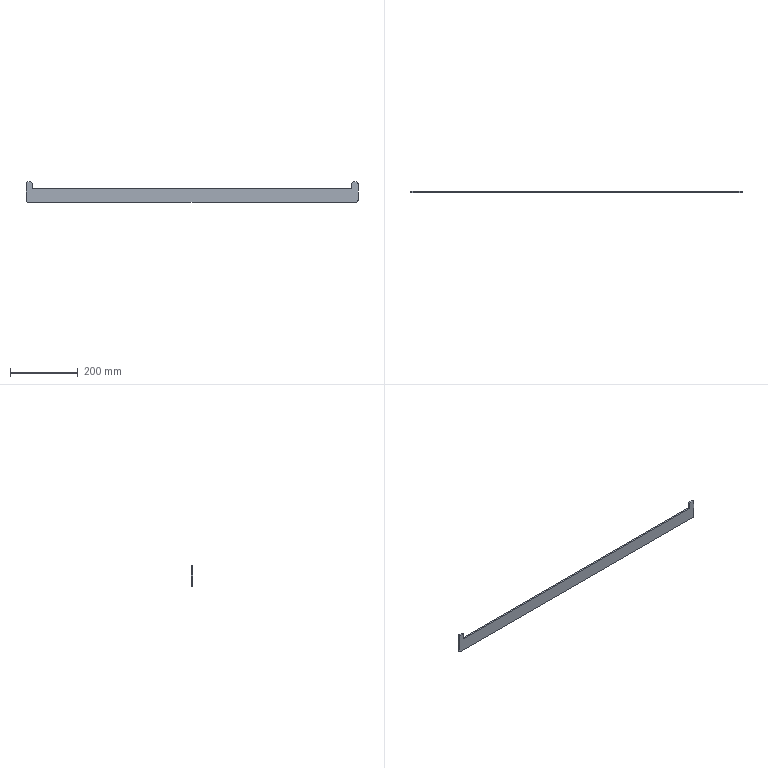Part | SolidWorks | features ICE 3, Fillet 2, FlatPattern 1, SMBaseFlange 1, SheetMetal 1 | 1 solid | 16 faces | box 980 x 5 x 60 mm | volume 199439 mm3 | plane 10 | cylinder 6 | commonest cylinder face diameters 10 x6
STEP:
#1=CARTESIAN_POINT('',(-472.,-5.,20.));
#2=VERTEX_POINT('',#1);
#3=CARTESIAN_POINT('',(-472.,0.,20.));
#4=VERTEX_POINT('',#3);
#5=CARTESIAN_POINT('',(-472.,-31.907,20.));
#6=DIRECTION('',(0.,1.,0.));
#7=VECTOR('',#6,1000.);
#8=LINE('',#5,#7);
#9=EDGE_CURVE('',#2,#4,#8,.T.);
#10=ORIENTED_EDGE('',*,*,#9,.F.);
#11=CARTESIAN_POINT('',(472.,-5.,20.));
#12=VERTEX_POINT('',#11);
#13=CARTESIAN_POINT('',(-490.,-5.,20.));
#14=DIRECTION('',(1.,0.,0.));
#15=VECTOR('',#14,1000.);
#16=LINE('',#13,#15);
#17=EDGE_CURVE('',#2,#12,#16,.T.);
#18=ORIENTED_EDGE('',*,*,#17,.T.);
#19=CARTESIAN_POINT('',(472.,0.,20.));
#20=VERTEX_POINT('',#19);
#21=CARTESIAN_POINT('',(472.,-5.,20.));
#22=DIRECTION('',(0.,1.,0.));
#23=VECTOR('',#22,1000.);
#24=LINE('',#21,#23);
#25=EDGE_CURVE('',#12,#20,#24,.T.);
#26=ORIENTED_EDGE('',*,*,#25,.T.);
#27=CARTESIAN_POINT('',(-490.,0.,20.));
#28=DIRECTION('',(1.,0.,0.));
#29=VECTOR('',#28,1000.);
#30=LINE('',#27,#29);
#31=EDGE_CURVE('',#4,#20,#30,.T.);
#32=ORIENTED_EDGE('',*,*,#31,.F.);
#33=EDGE_LOOP('',(#10,#18,#26,#32));
#34=FACE_OUTER_BOUND('',#33,.T.);
#35=CARTESIAN_POINT('',(-490.,-5.,20.));
#36=DIRECTION('',(0.,0.,1.));
#37=DIRECTION('',(1.,0.,0.));
#38=AXIS2_PLACEMENT_3D('',#35,#36,#37);
#39=PLANE('',#38);
#40=ADVANCED_FACE('',(#34),#39,.T.);
#41=CARTESIAN_POINT('',(490.,-5.,35.));
#42=VERTEX_POINT('',#41);
#43=CARTESIAN_POINT('',(490.,-5.,-15.));
#44=VERTEX_POINT('',#43);
#45=CARTESIAN_POINT('',(490.,-5.,20.));
#46=DIRECTION('',(0.,0.,-1.));
#47=VECTOR('',#46,1000.);
#48=LINE('',#45,#47);
#49=EDGE_CURVE('',#42,#44,#48,.T.);
#50=ORIENTED_EDGE('',*,*,#49,.T.);
#51=CARTESIAN_POINT('',(490.,0.,-15.));
#52=VERTEX_POINT('',#51);
#53=CARTESIAN_POINT('',(490.,-5.,-15.));
#54=DIRECTION('',(0.,1.,0.));
#55=VECTOR('',#54,1000.);
#56=LINE('',#53,#55);
#57=EDGE_CURVE('',#44,#52,#56,.T.);
#58=ORIENTED_EDGE('',*,*,#57,.T.);
#59=CARTESIAN_POINT('',(490.,0.,35.));
#60=VERTEX_POINT('',#59);
#61=CARTESIAN_POINT('',(490.,0.,20.));
#62=DIRECTION('',(0.,0.,-1.));
#63=VECTOR('',#62,1000.);
#64=LINE('',#61,#63);
#65=EDGE_CURVE('',#60,#52,#64,.T.);
#66=ORIENTED_EDGE('',*,*,#65,.F.);
#67=CARTESIAN_POINT('',(490.,-5.,35.));
#68=DIRECTION('',(0.,-1.,0.));
#69=VECTOR('',#68,1000.);
#70=LINE('',#67,#69);
#71=EDGE_CURVE('',#60,#42,#70,.T.);
#72=ORIENTED_EDGE('',*,*,#71,.T.);
#73=EDGE_LOOP('',(#50,#58,#66,#72));
#74=FACE_OUTER_BOUND('',#73,.T.);
#75=CARTESIAN_POINT('',(490.,-5.,20.));
#76=DIRECTION('',(1.,0.,0.));
#77=DIRECTION('',(0.,0.,-1.));
#78=AXIS2_PLACEMENT_3D('',#75,#76,#77);
#79=PLANE('',#78);
#80=ADVANCED_FACE('',(#74),#79,.T.);
#81=CARTESIAN_POINT('',(-490.,-5.,-15.));
#82=VERTEX_POINT('',#81);
#83=CARTESIAN_POINT('',(-490.,-5.,35.));
#84=VERTEX_POINT('',#83);
#85=CARTESIAN_POINT('',(-490.,-5.,20.));
#86=DIRECTION('',(0.,0.,1.));
#87=VECTOR('',#86,1000.);
#88=LINE('',#85,#87);
#89=EDGE_CURVE('',#82,#84,#88,.T.);
#90=ORIENTED_EDGE('',*,*,#89,.T.);
#91=CARTESIAN_POINT('',(-490.,0.,35.));
#92=VERTEX_POINT('',#91);
#93=CARTESIAN_POINT('',(-490.,-5.,35.));
#94=DIRECTION('',(0.,1.,0.));
#95=VECTOR('',#94,1000.);
#96=LINE('',#93,#95);
#97=EDGE_CURVE('',#84,#92,#96,.T.);
#98=ORIENTED_EDGE('',*,*,#97,.T.);
#99=CARTESIAN_POINT('',(-490.,0.,-15.));
#100=VERTEX_POINT('',#99);
#101=CARTESIAN_POINT('',(-490.,0.,20.));
#102=DIRECTION('',(0.,0.,1.));
#103=VECTOR('',#102,1000.);
#104=LINE('',#101,#103);
#105=EDGE_CURVE('',#100,#92,#104,.T.);
#106=ORIENTED_EDGE('',*,*,#105,.F.);
#107=CARTESIAN_POINT('',(-490.,-5.,-15.));
#108=DIRECTION('',(0.,-1.,0.));
#109=VECTOR('',#108,1000.);
#110=LINE('',#107,#109);
#111=EDGE_CURVE('',#100,#82,#110,.T.);
#112=ORIENTED_EDGE('',*,*,#111,.T.);
#113=EDGE_LOOP('',(#90,#98,#106,#112));
#114=FACE_OUTER_BOUND('',#113,.T.);
#115=CARTESIAN_POINT('',(-490.,-5.,20.));
#116=DIRECTION('',(-1.,0.,0.));
#117=DIRECTION('',(0.,0.,1.));
#118=AXIS2_PLACEMENT_3D('',#115,#116,#117);
#119=PLANE('',#118);
#120=ADVANCED_FACE('',(#114),#119,.T.);
#121=CARTESIAN_POINT('',(485.,0.,-20.));
#122=VERTEX_POINT('',#121);
#123=CARTESIAN_POINT('',(-485.,0.,-20.));
#124=VERTEX_POINT('',#123);
#125=CARTESIAN_POINT('',(-490.,0.,-20.));
#126=DIRECTION('',(-1.,0.,0.));
#127=VECTOR('',#126,1000.);
#128=LINE('',#125,#127);
#129=EDGE_CURVE('',#122,#124,#128,.T.);
#130=ORIENTED_EDGE('',*,*,#129,.F.);
#131=CARTESIAN_POINT('',(485.,-5.,-20.));
#132=VERTEX_POINT('',#131);
#133=CARTESIAN_POINT('',(485.,-5.,-20.));
#134=DIRECTION('',(0.,-1.,0.));
#135=VECTOR('',#134,1000.);
#136=LINE('',#133,#135);
#137=EDGE_CURVE('',#122,#132,#136,.T.);
#138=ORIENTED_EDGE('',*,*,#137,.T.);
#139=CARTESIAN_POINT('',(-485.,-5.,-20.));
#140=VERTEX_POINT('',#139);
#141=CARTESIAN_POINT('',(-490.,-5.,-20.));
#142=DIRECTION('',(-1.,0.,0.));
#143=VECTOR('',#142,1000.);
#144=LINE('',#141,#143);
#145=EDGE_CURVE('',#132,#140,#144,.T.);
#146=ORIENTED_EDGE('',*,*,#145,.T.);
#147=CARTESIAN_POINT('',(-485.,-5.,-20.));
#148=DIRECTION('',(0.,1.,0.));
#149=VECTOR('',#148,1000.);
#150=LINE('',#147,#149);
#151=EDGE_CURVE('',#140,#124,#150,.T.);
#152=ORIENTED_EDGE('',*,*,#151,.T.);
#153=EDGE_LOOP('',(#130,#138,#146,#152));
#154=FACE_OUTER_BOUND('',#153,.T.);
#155=CARTESIAN_POINT('',(-490.,-5.,-20.));
#156=DIRECTION('',(0.,0.,-1.));
#157=DIRECTION('',(-1.,0.,0.));
#158=AXIS2_PLACEMENT_3D('',#155,#156,#157);
#159=PLANE('',#158);
#160=ADVANCED_FACE('',(#154),#159,.T.);
#161=CARTESIAN_POINT('',(-472.,-5.,35.));
#162=VERTEX_POINT('',#161);
#163=CARTESIAN_POINT('',(-472.,-5.,20.));
#164=DIRECTION('',(0.,0.,-1.));
#165=VECTOR('',#164,1000.);
#166=LINE('',#163,#165);
#167=EDGE_CURVE('',#162,#2,#166,.T.);
#168=ORIENTED_EDGE('',*,*,#167,.F.);
#169=CARTESIAN_POINT('',(-477.,-5.,40.));
#170=VERTEX_POINT('',#169);
#171=CARTESIAN_POINT('',(-477.,-5.,35.));
#172=DIRECTION('',(0.,-1.,0.));
#173=DIRECTION('',(0.,0.,-1.));
#174=AXIS2_PLACEMENT_3D('',#171,#172,#173);
#175=CIRCLE('',#174,5.);
#176=EDGE_CURVE('',#162,#170,#175,.T.);
#177=ORIENTED_EDGE('',*,*,#176,.T.);
#178=CARTESIAN_POINT('',(-485.,-5.,40.));
#179=VERTEX_POINT('',#178);
#180=CARTESIAN_POINT('',(-490.,-5.,40.));
#181=DIRECTION('',(1.,0.,0.));
#182=VECTOR('',#181,1000.);
#183=LINE('',#180,#182);
#184=EDGE_CURVE('',#179,#170,#183,.T.);
#185=ORIENTED_EDGE('',*,*,#184,.F.);
#186=CARTESIAN_POINT('',(-485.,-5.,35.));
#187=DIRECTION('',(0.,-1.,0.));
#188=DIRECTION('',(0.,0.,-1.));
#189=AXIS2_PLACEMENT_3D('',#186,#187,#188);
#190=CIRCLE('',#189,5.);
#191=EDGE_CURVE('',#179,#84,#190,.T.);
#192=ORIENTED_EDGE('',*,*,#191,.T.);
#193=ORIENTED_EDGE('',*,*,#89,.F.);
#194=CARTESIAN_POINT('',(-485.,-5.,-15.));
#195=DIRECTION('',(0.,-1.,0.));
#196=DIRECTION('',(0.,0.,-1.));
#197=AXIS2_PLACEMENT_3D('',#194,#195,#196);
#198=CIRCLE('',#197,5.);
#199=EDGE_CURVE('',#82,#140,#198,.T.);
#200=ORIENTED_EDGE('',*,*,#199,.T.);
#201=ORIENTED_EDGE('',*,*,#145,.F.);
#202=CARTESIAN_POINT('',(485.,-5.,-15.));
#203=DIRECTION('',(0.,-1.,0.));
#204=DIRECTION('',(0.,0.,-1.));
#205=AXIS2_PLACEMENT_3D('',#202,#203,#204);
#206=CIRCLE('',#205,5.);
#207=EDGE_CURVE('',#132,#44,#206,.T.);
#208=ORIENTED_EDGE('',*,*,#207,.T.);
#209=ORIENTED_EDGE('',*,*,#49,.F.);
#210=CARTESIAN_POINT('',(485.,-5.,40.));
#211=VERTEX_POINT('',#210);
#212=CARTESIAN_POINT('',(485.,-5.,35.));
#213=DIRECTION('',(0.,-1.,0.));
#214=DIRECTION('',(0.,0.,-1.));
#215=AXIS2_PLACEMENT_3D('',#212,#213,#214);
#216=CIRCLE('',#215,5.);
#217=EDGE_CURVE('',#42,#211,#216,.T.);
#218=ORIENTED_EDGE('',*,*,#217,.T.);
#219=CARTESIAN_POINT('',(477.,-5.,40.));
#220=VERTEX_POINT('',#219);
#221=CARTESIAN_POINT('',(490.,-5.,40.));
#222=DIRECTION('',(1.,0.,0.));
#223=VECTOR('',#222,1000.);
#224=LINE('',#221,#223);
#225=EDGE_CURVE('',#220,#211,#224,.T.);
#226=ORIENTED_EDGE('',*,*,#225,.F.);
#227=CARTESIAN_POINT('',(472.,-5.,35.));
#228=VERTEX_POINT('',#227);
#229=CARTESIAN_POINT('',(477.,-5.,35.));
#230=DIRECTION('',(0.,-1.,0.));
#231=DIRECTION('',(0.,0.,-1.));
#232=AXIS2_PLACEMENT_3D('',#229,#230,#231);
#233=CIRCLE('',#232,5.);
#234=EDGE_CURVE('',#220,#228,#233,.T.);
#235=ORIENTED_EDGE('',*,*,#234,.T.);
#236=CARTESIAN_POINT('',(472.,-5.,20.));
#237=DIRECTION('',(0.,0.,1.));
#238=VECTOR('',#237,1000.);
#239=LINE('',#236,#238);
#240=EDGE_CURVE('',#12,#228,#239,.T.);
#241=ORIENTED_EDGE('',*,*,#240,.F.);
#242=ORIENTED_EDGE('',*,*,#17,.F.);
#243=EDGE_LOOP('',(#168,#177,#185,#192,#193,#200,#201,#208,#209,#218,#226,#235,#241,#242));
#244=FACE_OUTER_BOUND('',#243,.T.);
#245=CARTESIAN_POINT('',(0.,-5.,0.));
#246=DIRECTION('',(0.,-1.,0.));
#247=DIRECTION('',(0.,0.,-1.));
#248=AXIS2_PLACEMENT_3D('',#245,#246,#247);
#249=PLANE('',#248);
#250=ADVANCED_FACE('',(#244),#249,.T.);
#251=CARTESIAN_POINT('',(-485.,0.,40.));
#252=VERTEX_POINT('',#251);
#253=CARTESIAN_POINT('',(-477.,0.,40.));
#254=VERTEX_POINT('',#253);
#255=CARTESIAN_POINT('',(-490.,0.,40.));
#256=DIRECTION('',(1.,0.,0.));
#257=VECTOR('',#256,1000.);
#258=LINE('',#255,#257);
#259=EDGE_CURVE('',#252,#254,#258,.T.);
#260=ORIENTED_EDGE('',*,*,#259,.T.);
#261=CARTESIAN_POINT('',(-472.,0.,35.));
#262=VERTEX_POINT('',#261);
#263=CARTESIAN_POINT('',(-477.,0.,35.));
#264=DIRECTION('',(0.,1.,0.));
#265=DIRECTION('',(0.,0.,-1.));
#266=AXIS2_PLACEMENT_3D('',#263,#264,#265);
#267=CIRCLE('',#266,5.);
#268=EDGE_CURVE('',#254,#262,#267,.T.);
#269=ORIENTED_EDGE('',*,*,#268,.T.);
#270=CARTESIAN_POINT('',(-472.,0.,20.));
#271=DIRECTION('',(0.,0.,-1.));
#272=VECTOR('',#271,1000.);
#273=LINE('',#270,#272);
#274=EDGE_CURVE('',#262,#4,#273,.T.);
#275=ORIENTED_EDGE('',*,*,#274,.T.);
#276=ORIENTED_EDGE('',*,*,#31,.T.);
#277=CARTESIAN_POINT('',(472.,0.,35.));
#278=VERTEX_POINT('',#277);
#279=CARTESIAN_POINT('',(472.,0.,20.));
#280=DIRECTION('',(0.,0.,1.));
#281=VECTOR('',#280,1000.);
#282=LINE('',#279,#281);
#283=EDGE_CURVE('',#20,#278,#282,.T.);
#284=ORIENTED_EDGE('',*,*,#283,.T.);
#285=CARTESIAN_POINT('',(477.,0.,40.));
#286=VERTEX_POINT('',#285);
#287=CARTESIAN_POINT('',(477.,0.,35.));
#288=DIRECTION('',(0.,1.,0.));
#289=DIRECTION('',(0.,0.,-1.));
#290=AXIS2_PLACEMENT_3D('',#287,#288,#289);
#291=CIRCLE('',#290,5.);
#292=EDGE_CURVE('',#278,#286,#291,.T.);
#293=ORIENTED_EDGE('',*,*,#292,.T.);
#294=CARTESIAN_POINT('',(485.,0.,40.));
#295=VERTEX_POINT('',#294);
#296=CARTESIAN_POINT('',(490.,0.,40.));
#297=DIRECTION('',(1.,0.,0.));
#298=VECTOR('',#297,1000.);
#299=LINE('',#296,#298);
#300=EDGE_CURVE('',#286,#295,#299,.T.);
#301=ORIENTED_EDGE('',*,*,#300,.T.);
#302=CARTESIAN_POINT('',(485.,0.,35.));
#303=DIRECTION('',(0.,1.,0.));
#304=DIRECTION('',(0.,0.,-1.));
#305=AXIS2_PLACEMENT_3D('',#302,#303,#304);
#306=CIRCLE('',#305,5.);
#307=EDGE_CURVE('',#295,#60,#306,.T.);
#308=ORIENTED_EDGE('',*,*,#307,.T.);
#309=ORIENTED_EDGE('',*,*,#65,.T.);
#310=CARTESIAN_POINT('',(485.,0.,-15.));
#311=DIRECTION('',(0.,1.,0.));
#312=DIRECTION('',(0.,0.,-1.));
#313=AXIS2_PLACEMENT_3D('',#310,#311,#312);
#314=CIRCLE('',#313,5.);
#315=EDGE_CURVE('',#52,#122,#314,.T.);
#316=ORIENTED_EDGE('',*,*,#315,.T.);
#317=ORIENTED_EDGE('',*,*,#129,.T.);
#318=CARTESIAN_POINT('',(-485.,0.,-15.));
#319=DIRECTION('',(0.,1.,0.));
#320=DIRECTION('',(0.,0.,-1.));
#321=AXIS2_PLACEMENT_3D('',#318,#319,#320);
#322=CIRCLE('',#321,5.);
#323=EDGE_CURVE('',#124,#100,#322,.T.);
#324=ORIENTED_EDGE('',*,*,#323,.T.);
#325=ORIENTED_EDGE('',*,*,#105,.T.);
#326=CARTESIAN_POINT('',(-485.,0.,35.));
#327=DIRECTION('',(0.,1.,0.));
#328=DIRECTION('',(0.,0.,-1.));
#329=AXIS2_PLACEMENT_3D('',#326,#327,#328);
#330=CIRCLE('',#329,5.);
#331=EDGE_CURVE('',#92,#252,#330,.T.);
#332=ORIENTED_EDGE('',*,*,#331,.T.);
#333=EDGE_LOOP('',(#260,#269,#275,#276,#284,#293,#301,#308,#309,#316,#317,#324,#325,#332));
#334=FACE_OUTER_BOUND('',#333,.T.);
#335=CARTESIAN_POINT('',(0.,0.,0.));
#336=DIRECTION('',(0.,-1.,0.));
#337=DIRECTION('',(0.,0.,-1.));
#338=AXIS2_PLACEMENT_3D('',#335,#336,#337);
#339=PLANE('',#338);
#340=ADVANCED_FACE('',(#334),#339,.F.);
#341=ORIENTED_EDGE('',*,*,#225,.T.);
#342=CARTESIAN_POINT('',(485.,-5.,40.));
#343=DIRECTION('',(0.,1.,0.));
#344=VECTOR('',#343,1000.);
#345=LINE('',#342,#344);
#346=EDGE_CURVE('',#211,#295,#345,.T.);
#347=ORIENTED_EDGE('',*,*,#346,.T.);
#348=ORIENTED_EDGE('',*,*,#300,.F.);
#349=CARTESIAN_POINT('',(477.,-5.,40.));
#350=DIRECTION('',(0.,-1.,0.));
#351=VECTOR('',#350,1000.);
#352=LINE('',#349,#351);
#353=EDGE_CURVE('',#286,#220,#352,.T.);
#354=ORIENTED_EDGE('',*,*,#353,.T.);
#355=EDGE_LOOP('',(#341,#347,#348,#354));
#356=FACE_OUTER_BOUND('',#355,.T.);
#357=CARTESIAN_POINT('',(490.,-5.,40.));
#358=DIRECTION('',(0.,0.,1.));
#359=DIRECTION('',(1.,0.,0.));
#360=AXIS2_PLACEMENT_3D('',#357,#358,#359);
#361=PLANE('',#360);
#362=ADVANCED_FACE('',(#356),#361,.T.);
#363=ORIENTED_EDGE('',*,*,#240,.T.);
#364=CARTESIAN_POINT('',(472.,-5.,35.));
#365=DIRECTION('',(0.,1.,0.));
#366=VECTOR('',#365,1000.);
#367=LINE('',#364,#366);
#368=EDGE_CURVE('',#228,#278,#367,.T.);
#369=ORIENTED_EDGE('',*,*,#368,.T.);
#370=ORIENTED_EDGE('',*,*,#283,.F.);
#371=ORIENTED_EDGE('',*,*,#25,.F.);
#372=EDGE_LOOP('',(#363,#369,#370,#371));
#373=FACE_OUTER_BOUND('',#372,.T.);
#374=CARTESIAN_POINT('',(472.,-5.,20.));
#375=DIRECTION('',(-1.,0.,0.));
#376=DIRECTION('',(0.,0.,1.));
#377=AXIS2_PLACEMENT_3D('',#374,#375,#376);
#378=PLANE('',#377);
#379=ADVANCED_FACE('',(#373),#378,.T.);
#380=ORIENTED_EDGE('',*,*,#207,.F.);
#381=ORIENTED_EDGE('',*,*,#137,.F.);
#382=ORIENTED_EDGE('',*,*,#315,.F.);
#383=ORIENTED_EDGE('',*,*,#57,.F.);
#384=EDGE_LOOP('',(#380,#381,#382,#383));
#385=FACE_OUTER_BOUND('',#384,.T.);
#386=CARTESIAN_POINT('',(485.,-5.,-15.));
#387=DIRECTION('',(0.,1.,0.));
#388=DIRECTION('',(0.,0.,1.));
#389=AXIS2_PLACEMENT_3D('',#386,#387,#388);
#390=CYLINDRICAL_SURFACE('',#389,5.);
#391=ADVANCED_FACE('',(#385),#390,.T.);
#392=ORIENTED_EDGE('',*,*,#199,.F.);
#393=ORIENTED_EDGE('',*,*,#111,.F.);
#394=ORIENTED_EDGE('',*,*,#323,.F.);
#395=ORIENTED_EDGE('',*,*,#151,.F.);
#396=EDGE_LOOP('',(#392,#393,#394,#395));
#397=FACE_OUTER_BOUND('',#396,.T.);
#398=CARTESIAN_POINT('',(-485.,-5.,-15.));
#399=DIRECTION('',(0.,1.,0.));
#400=DIRECTION('',(0.,0.,1.));
#401=AXIS2_PLACEMENT_3D('',#398,#399,#400);
#402=CYLINDRICAL_SURFACE('',#401,5.);
#403=ADVANCED_FACE('',(#397),#402,.T.);
#404=ORIENTED_EDGE('',*,*,#217,.F.);
#405=ORIENTED_EDGE('',*,*,#71,.F.);
#406=ORIENTED_EDGE('',*,*,#307,.F.);
#407=ORIENTED_EDGE('',*,*,#346,.F.);
#408=EDGE_LOOP('',(#404,#405,#406,#407));
#409=FACE_OUTER_BOUND('',#408,.T.);
#410=CARTESIAN_POINT('',(485.,-5.,35.));
#411=DIRECTION('',(0.,1.,0.));
#412=DIRECTION('',(0.,0.,1.));
#413=AXIS2_PLACEMENT_3D('',#410,#411,#412);
#414=CYLINDRICAL_SURFACE('',#413,5.);
#415=ADVANCED_FACE('',(#409),#414,.T.);
#416=ORIENTED_EDGE('',*,*,#234,.F.);
#417=ORIENTED_EDGE('',*,*,#353,.F.);
#418=ORIENTED_EDGE('',*,*,#292,.F.);
#419=ORIENTED_EDGE('',*,*,#368,.F.);
#420=EDGE_LOOP('',(#416,#417,#418,#419));
#421=FACE_OUTER_BOUND('',#420,.T.);
#422=CARTESIAN_POINT('',(477.,-5.,35.));
#423=DIRECTION('',(0.,1.,0.));
#424=DIRECTION('',(0.,0.,1.));
#425=AXIS2_PLACEMENT_3D('',#422,#423,#424);
#426=CYLINDRICAL_SURFACE('',#425,5.);
#427=ADVANCED_FACE('',(#421),#426,.T.);
#428=ORIENTED_EDGE('',*,*,#184,.T.);
#429=CARTESIAN_POINT('',(-477.,-31.907,40.));
#430=DIRECTION('',(0.,1.,0.));
#431=VECTOR('',#430,1000.);
#432=LINE('',#429,#431);
#433=EDGE_CURVE('',#170,#254,#432,.T.);
#434=ORIENTED_EDGE('',*,*,#433,.T.);
#435=ORIENTED_EDGE('',*,*,#259,.F.);
#436=CARTESIAN_POINT('',(-485.,-31.907,40.));
#437=DIRECTION('',(0.,-1.,0.));
#438=VECTOR('',#437,1000.);
#439=LINE('',#436,#438);
#440=EDGE_CURVE('',#252,#179,#439,.T.);
#441=ORIENTED_EDGE('',*,*,#440,.T.);
#442=EDGE_LOOP('',(#428,#434,#435,#441));
#443=FACE_OUTER_BOUND('',#442,.T.);
#444=CARTESIAN_POINT('',(-490.,-31.907,40.));
#445=DIRECTION('',(0.,0.,1.));
#446=DIRECTION('',(1.,0.,0.));
#447=AXIS2_PLACEMENT_3D('',#444,#445,#446);
#448=PLANE('',#447);
#449=ADVANCED_FACE('',(#443),#448,.T.);
#450=ORIENTED_EDGE('',*,*,#274,.F.);
#451=CARTESIAN_POINT('',(-472.,-31.907,35.));
#452=DIRECTION('',(0.,-1.,0.));
#453=VECTOR('',#452,1000.);
#454=LINE('',#451,#453);
#455=EDGE_CURVE('',#262,#162,#454,.T.);
#456=ORIENTED_EDGE('',*,*,#455,.T.);
#457=ORIENTED_EDGE('',*,*,#167,.T.);
#458=ORIENTED_EDGE('',*,*,#9,.T.);
#459=EDGE_LOOP('',(#450,#456,#457,#458));
#460=FACE_OUTER_BOUND('',#459,.T.);
#461=CARTESIAN_POINT('',(-472.,-31.907,20.));
#462=DIRECTION('',(1.,0.,0.));
#463=DIRECTION('',(0.,0.,-1.));
#464=AXIS2_PLACEMENT_3D('',#461,#462,#463);
#465=PLANE('',#464);
#466=ADVANCED_FACE('',(#460),#465,.T.);
#467=ORIENTED_EDGE('',*,*,#176,.F.);
#468=ORIENTED_EDGE('',*,*,#455,.F.);
#469=ORIENTED_EDGE('',*,*,#268,.F.);
#470=ORIENTED_EDGE('',*,*,#433,.F.);
#471=EDGE_LOOP('',(#467,#468,#469,#470));
#472=FACE_OUTER_BOUND('',#471,.T.);
#473=CARTESIAN_POINT('',(-477.,-31.907,35.));
#474=DIRECTION('',(0.,1.,0.));
#475=DIRECTION('',(0.,0.,1.));
#476=AXIS2_PLACEMENT_3D('',#473,#474,#475);
#477=CYLINDRICAL_SURFACE('',#476,5.);
#478=ADVANCED_FACE('',(#472),#477,.T.);
#479=ORIENTED_EDGE('',*,*,#191,.F.);
#480=ORIENTED_EDGE('',*,*,#440,.F.);
#481=ORIENTED_EDGE('',*,*,#331,.F.);
#482=ORIENTED_EDGE('',*,*,#97,.F.);
#483=EDGE_LOOP('',(#479,#480,#481,#482));
#484=FACE_OUTER_BOUND('',#483,.T.);
#485=CARTESIAN_POINT('',(-485.,-5.,35.));
#486=DIRECTION('',(0.,1.,0.));
#487=DIRECTION('',(0.,0.,1.));
#488=AXIS2_PLACEMENT_3D('',#485,#486,#487);
#489=CYLINDRICAL_SURFACE('',#488,5.);
#490=ADVANCED_FACE('',(#484),#489,.T.);
#491=CLOSED_SHELL('',(#40,#80,#120,#160,#250,#340,#362,#379,#391,#403,#415,#427,#449,#466,#478,#490));
#492=MANIFOLD_SOLID_BREP('',#491);
#493=CARTESIAN_POINT('',(0.,0.,0.));
#494=DIRECTION('',(0.,0.,1.));
#495=DIRECTION('',(1.,0.,0.));
#496=AXIS2_PLACEMENT_3D('',#493,#494,#495);
#497=(LENGTH_UNIT()NAMED_UNIT(*)SI_UNIT(.MILLI.,.METRE.));
#498=UNCERTAINTY_MEASURE_WITH_UNIT(LENGTH_MEASURE(0.00001),#497,'','');
#499=(NAMED_UNIT(*)PLANE_ANGLE_UNIT()SI_UNIT($,.RADIAN.));
#500=(NAMED_UNIT(*)SI_UNIT($,.STERADIAN.)SOLID_ANGLE_UNIT());
#501=(GEOMETRIC_REPRESENTATION_CONTEXT(3)GLOBAL_UNCERTAINTY_ASSIGNED_CONTEXT((#498))GLOBAL_UNIT_ASSIGNED_CONTEXT((#497,#499,#500))REPRESENTATION_CONTEXT('',''));
#502=ADVANCED_BREP_SHAPE_REPRESENTATION('',(#492,#496),#501);